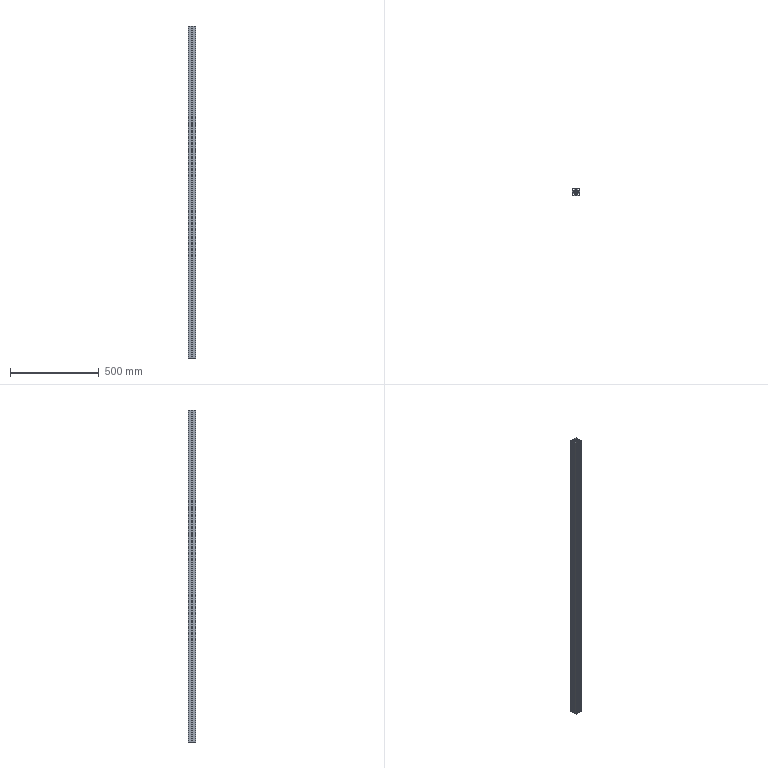Part | STEP file | 40_40_3240_1-2 | 1 solid | 64 faces | box 40 x 40 x 1875 mm | volume 983893 mm3 | plane 62 | cylinder 2 | commonest cylinder face diameters 6.8 x2